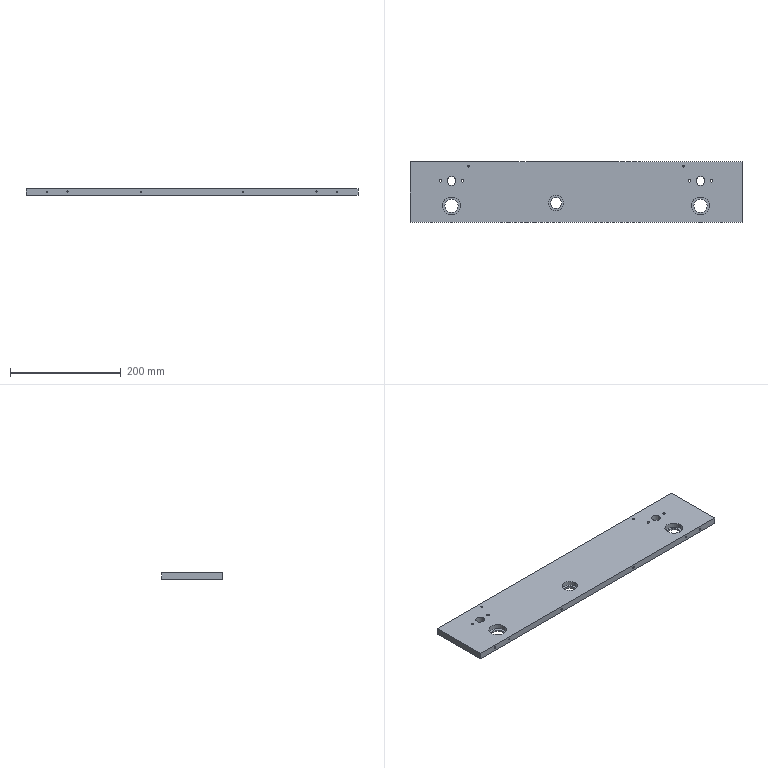Part | SolidWorks | features ICE 5, HoleWzd 4, Extrusion 1 | 1 solid | 57 faces | box 600 x 110 x 12 mm | volume 762368 mm3 | cylinder 40 | plane 9 | cone 8 | commonest cylinder face diameters 3.3 x12 4.2 x8 2.5 x4 16 x4 24 x4 32 x4